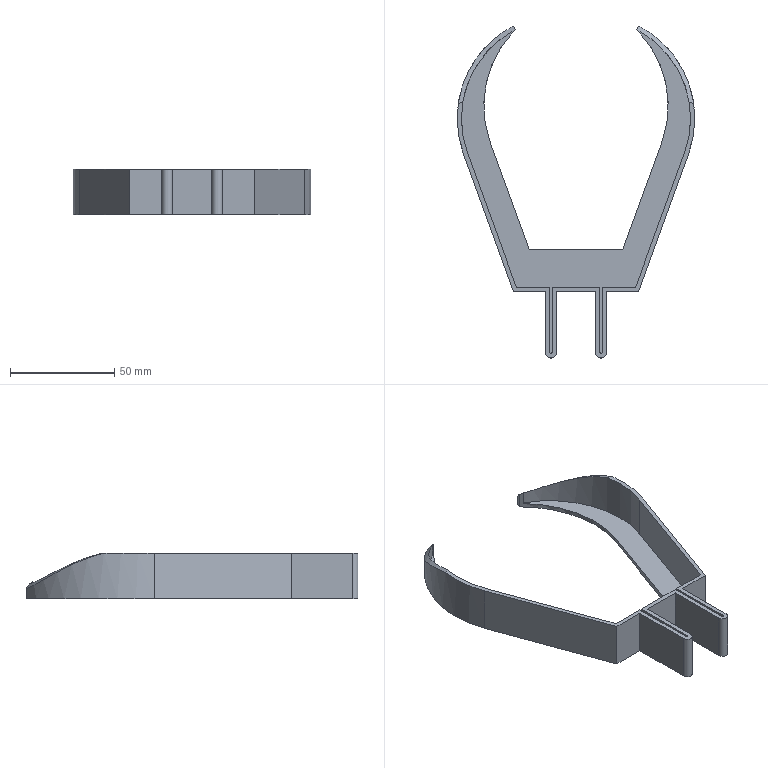Part | NX | features EXTRUDE 3, DATUM_CSYS 2, EXTRACT_STRING 2, SKETCH 2, Instance Feature 1, Mirror Feature 1, SHELL 1 | 1 solid | 40 faces | box 113.914 x 159.253 x 22 mm | volume 25744 mm3 | plane 28 | cylinder 12 | commonest cylinder face diameters 1 x2 5 x2 96 x2 100 x2 102.897 x2 103.017 x2
STEP:
#1=CARTESIAN_POINT('',(30.,127.253,4.945));
#2=VERTEX_POINT('',#1);
#3=CARTESIAN_POINT('',(29.078,125.478,7.237));
#4=VERTEX_POINT('',#3);
#5=CARTESIAN_POINT('',(11.445,91.523,-27.603));
#6=DIRECTION('',(-0.8875,0.4609,0.));
#7=DIRECTION('',(0.4609,0.8875,0.));
#8=AXIS2_PLACEMENT_3D('',#5,#6,#7);
#9=ELLIPSE('',#8,51.946,51.508);
#10=EDGE_CURVE('',#2,#4,#9,.F.);
#11=ORIENTED_EDGE('',*,*,#10,.F.);
#12=CARTESIAN_POINT('',(30.,127.253,0.));
#13=VERTEX_POINT('',#12);
#14=CARTESIAN_POINT('',(30.,127.253,22.));
#15=DIRECTION('',(0.,0.,-1.));
#16=VECTOR('',#15,1000.);
#17=LINE('',#14,#16);
#18=EDGE_CURVE('',#2,#13,#17,.T.);
#19=ORIENTED_EDGE('',*,*,#18,.T.);
#20=CARTESIAN_POINT('',(29.078,125.478,0.));
#21=VERTEX_POINT('',#20);
#22=CARTESIAN_POINT('',(29.078,125.478,0.));
#23=DIRECTION('',(0.4609,0.8875,0.));
#24=VECTOR('',#23,1000.);
#25=LINE('',#22,#24);
#26=EDGE_CURVE('',#21,#13,#25,.T.);
#27=ORIENTED_EDGE('',*,*,#26,.F.);
#28=CARTESIAN_POINT('',(29.078,125.478,22.));
#29=DIRECTION('',(0.,0.,-1.));
#30=VECTOR('',#29,1000.);
#31=LINE('',#28,#30);
#32=EDGE_CURVE('',#4,#21,#31,.T.);
#33=ORIENTED_EDGE('',*,*,#32,.F.);
#34=EDGE_LOOP('',(#11,#19,#27,#33));
#35=FACE_BOUND('',#34,.T.);
#36=CARTESIAN_POINT('',(29.078,125.478,22.));
#37=DIRECTION('',(-0.8875,0.4609,0.));
#38=DIRECTION('',(-0.4609,-0.8875,0.));
#39=AXIS2_PLACEMENT_3D('',#36,#37,#38);
#40=PLANE('',#39);
#41=ADVANCED_FACE('',(#35),#40,.T.);
#42=CARTESIAN_POINT('',(30.834,124.519,7.561));
#43=VERTEX_POINT('',#42);
#44=CARTESIAN_POINT('',(30.834,124.519,2.));
#45=VERTEX_POINT('',#44);
#46=CARTESIAN_POINT('',(30.834,124.519,22.));
#47=DIRECTION('',(0.,0.,-1.));
#48=VECTOR('',#47,1000.);
#49=LINE('',#46,#48);
#50=EDGE_CURVE('',#43,#45,#49,.T.);
#51=ORIENTED_EDGE('',*,*,#50,.F.);
#52=CARTESIAN_POINT('',(30.543,123.959,8.219));
#53=VERTEX_POINT('',#52);
#54=CARTESIAN_POINT('',(13.341,90.833,-27.603));
#55=DIRECTION('',(-0.8875,0.4609,0.));
#56=DIRECTION('',(0.4609,0.8875,0.));
#57=AXIS2_PLACEMENT_3D('',#54,#55,#56);
#58=ELLIPSE('',#57,51.946,51.508);
#59=EDGE_CURVE('',#43,#53,#58,.F.);
#60=ORIENTED_EDGE('',*,*,#59,.T.);
#61=CARTESIAN_POINT('',(30.543,123.959,2.));
#62=VERTEX_POINT('',#61);
#63=CARTESIAN_POINT('',(30.543,123.959,22.));
#64=DIRECTION('',(0.,0.,-1.));
#65=VECTOR('',#64,1000.);
#66=LINE('',#63,#65);
#67=EDGE_CURVE('',#53,#62,#66,.T.);
#68=ORIENTED_EDGE('',*,*,#67,.T.);
#69=CARTESIAN_POINT('',(5.777,76.267,2.));
#70=DIRECTION('',(0.4609,0.8875,0.));
#71=VECTOR('',#70,1000.);
#72=LINE('',#69,#71);
#73=EDGE_CURVE('',#62,#45,#72,.T.);
#74=ORIENTED_EDGE('',*,*,#73,.T.);
#75=EDGE_LOOP('',(#51,#60,#68,#74));
#76=FACE_BOUND('',#75,.T.);
#77=CARTESIAN_POINT('',(30.853,124.556,22.));
#78=DIRECTION('',(-0.8875,0.4609,0.));
#79=DIRECTION('',(-0.4609,-0.8875,0.));
#80=AXIS2_PLACEMENT_3D('',#77,#78,#79);
#81=PLANE('',#80);
#82=ADVANCED_FACE('',(#76),#81,.F.);
#83=CARTESIAN_POINT('',(-29.078,125.478,7.237));
#84=VERTEX_POINT('',#83);
#85=CARTESIAN_POINT('',(-30.,127.253,4.945));
#86=VERTEX_POINT('',#85);
#87=CARTESIAN_POINT('',(-11.445,91.523,-27.603));
#88=DIRECTION('',(0.8875,0.4609,0.));
#89=DIRECTION('',(-0.4609,0.8875,0.));
#90=AXIS2_PLACEMENT_3D('',#87,#88,#89);
#91=ELLIPSE('',#90,51.946,51.508);
#92=EDGE_CURVE('',#84,#86,#91,.F.);
#93=ORIENTED_EDGE('',*,*,#92,.F.);
#94=CARTESIAN_POINT('',(-29.078,125.478,0.));
#95=VERTEX_POINT('',#94);
#96=CARTESIAN_POINT('',(-29.078,125.478,22.));
#97=DIRECTION('',(0.,0.,-1.));
#98=VECTOR('',#97,1000.);
#99=LINE('',#96,#98);
#100=EDGE_CURVE('',#84,#95,#99,.T.);
#101=ORIENTED_EDGE('',*,*,#100,.T.);
#102=CARTESIAN_POINT('',(-30.,127.253,0.));
#103=VERTEX_POINT('',#102);
#104=CARTESIAN_POINT('',(-30.,127.253,0.));
#105=DIRECTION('',(0.4609,-0.8875,0.));
#106=VECTOR('',#105,1000.);
#107=LINE('',#104,#106);
#108=EDGE_CURVE('',#103,#95,#107,.T.);
#109=ORIENTED_EDGE('',*,*,#108,.F.);
#110=CARTESIAN_POINT('',(-30.,127.253,22.));
#111=DIRECTION('',(0.,0.,-1.));
#112=VECTOR('',#111,1000.);
#113=LINE('',#110,#112);
#114=EDGE_CURVE('',#86,#103,#113,.T.);
#115=ORIENTED_EDGE('',*,*,#114,.F.);
#116=EDGE_LOOP('',(#93,#101,#109,#115));
#117=FACE_BOUND('',#116,.T.);
#118=CARTESIAN_POINT('',(-30.,127.253,22.));
#119=DIRECTION('',(0.8875,0.4609,0.));
#120=DIRECTION('',(-0.4609,0.8875,0.));
#121=AXIS2_PLACEMENT_3D('',#118,#119,#120);
#122=PLANE('',#121);
#123=ADVANCED_FACE('',(#117),#122,.T.);
#124=CARTESIAN_POINT('',(-30.543,123.959,8.219));
#125=VERTEX_POINT('',#124);
#126=CARTESIAN_POINT('',(-30.543,123.959,2.));
#127=VERTEX_POINT('',#126);
#128=CARTESIAN_POINT('',(-30.543,123.959,22.));
#129=DIRECTION('',(0.,0.,-1.));
#130=VECTOR('',#129,1000.);
#131=LINE('',#128,#130);
#132=EDGE_CURVE('',#125,#127,#131,.T.);
#133=ORIENTED_EDGE('',*,*,#132,.F.);
#134=CARTESIAN_POINT('',(-30.834,124.519,7.561));
#135=VERTEX_POINT('',#134);
#136=CARTESIAN_POINT('',(-13.341,90.833,-27.603));
#137=DIRECTION('',(0.8875,0.4609,0.));
#138=DIRECTION('',(-0.4609,0.8875,0.));
#139=AXIS2_PLACEMENT_3D('',#136,#137,#138);
#140=ELLIPSE('',#139,51.946,51.508);
#141=EDGE_CURVE('',#125,#135,#140,.F.);
#142=ORIENTED_EDGE('',*,*,#141,.T.);
#143=CARTESIAN_POINT('',(-30.834,124.519,2.));
#144=VERTEX_POINT('',#143);
#145=CARTESIAN_POINT('',(-30.834,124.519,22.));
#146=DIRECTION('',(0.,0.,-1.));
#147=VECTOR('',#146,1000.);
#148=LINE('',#145,#147);
#149=EDGE_CURVE('',#135,#144,#148,.T.);
#150=ORIENTED_EDGE('',*,*,#149,.T.);
#151=CARTESIAN_POINT('',(-8.732,81.958,2.));
#152=DIRECTION('',(0.4609,-0.8875,0.));
#153=VECTOR('',#152,1000.);
#154=LINE('',#151,#153);
#155=EDGE_CURVE('',#144,#127,#154,.T.);
#156=ORIENTED_EDGE('',*,*,#155,.T.);
#157=EDGE_LOOP('',(#133,#142,#150,#156));
#158=FACE_BOUND('',#157,.T.);
#159=CARTESIAN_POINT('',(-31.775,126.331,22.));
#160=DIRECTION('',(0.8875,0.4609,0.));
#161=DIRECTION('',(-0.4609,0.8875,0.));
#162=AXIS2_PLACEMENT_3D('',#159,#160,#161);
#163=PLANE('',#162);
#164=ADVANCED_FACE('',(#158),#163,.F.);
#165=CARTESIAN_POINT('',(-30.543,123.959,8.219));
#166=CARTESIAN_POINT('',(-30.068,124.473,7.889));
#167=CARTESIAN_POINT('',(-29.58,124.979,7.561));
#168=CARTESIAN_POINT('',(-29.078,125.478,7.237));
#169=B_SPLINE_CURVE_WITH_KNOTS('',3,(#165,#166,#167,#168),.UNSPECIFIED.,.F.,.F.,(4,4),(0.0356,0.0379),.UNSPECIFIED.);
#170=EDGE_CURVE('',#125,#84,#169,.T.);
#171=ORIENTED_EDGE('',*,*,#170,.F.);
#172=ORIENTED_EDGE('',*,*,#132,.T.);
#173=CARTESIAN_POINT('',(-41.696,73.068,2.));
#174=VERTEX_POINT('',#173);
#175=CARTESIAN_POINT('',(7.219,89.016,2.));
#176=DIRECTION('',(0.,0.,-1.));
#177=DIRECTION('',(-1.,0.,0.));
#178=AXIS2_PLACEMENT_3D('',#175,#176,#177);
#179=CIRCLE('',#178,51.449);
#180=EDGE_CURVE('',#127,#174,#179,.F.);
#181=ORIENTED_EDGE('',*,*,#180,.T.);
#182=CARTESIAN_POINT('',(-41.696,73.068,0.));
#183=VERTEX_POINT('',#182);
#184=CARTESIAN_POINT('',(-41.696,73.068,22.));
#185=DIRECTION('',(0.,0.,-1.));
#186=VECTOR('',#185,1000.);
#187=LINE('',#184,#186);
#188=EDGE_CURVE('',#174,#183,#187,.T.);
#189=ORIENTED_EDGE('',*,*,#188,.T.);
#190=CARTESIAN_POINT('',(7.219,89.016,0.));
#191=DIRECTION('',(0.,0.,1.));
#192=DIRECTION('',(-1.,0.,0.));
#193=AXIS2_PLACEMENT_3D('',#190,#191,#192);
#194=CIRCLE('',#193,51.449);
#195=EDGE_CURVE('',#95,#183,#194,.T.);
#196=ORIENTED_EDGE('',*,*,#195,.F.);
#197=ORIENTED_EDGE('',*,*,#100,.F.);
#198=EDGE_LOOP('',(#171,#172,#181,#189,#196,#197));
#199=FACE_BOUND('',#198,.T.);
#200=CARTESIAN_POINT('',(7.219,89.016,22.));
#201=DIRECTION('',(0.,0.,-1.));
#202=DIRECTION('',(-1.,0.,0.));
#203=AXIS2_PLACEMENT_3D('',#200,#201,#202);
#204=CYLINDRICAL_SURFACE('',#203,51.449);
#205=ADVANCED_FACE('',(#199),#204,.F.);
#206=ORIENTED_EDGE('',*,*,#188,.F.);
#207=CARTESIAN_POINT('',(-22.381,20.,2.));
#208=VERTEX_POINT('',#207);
#209=CARTESIAN_POINT('',(-40.786,70.567,2.));
#210=DIRECTION('',(0.342,-0.9397,0.));
#211=VECTOR('',#210,1000.);
#212=LINE('',#209,#211);
#213=EDGE_CURVE('',#174,#208,#212,.T.);
#214=ORIENTED_EDGE('',*,*,#213,.T.);
#215=CARTESIAN_POINT('',(-22.381,20.,0.));
#216=VERTEX_POINT('',#215);
#217=CARTESIAN_POINT('',(-22.381,20.,22.));
#218=DIRECTION('',(0.,0.,-1.));
#219=VECTOR('',#218,1000.);
#220=LINE('',#217,#219);
#221=EDGE_CURVE('',#208,#216,#220,.T.);
#222=ORIENTED_EDGE('',*,*,#221,.T.);
#223=CARTESIAN_POINT('',(-41.696,73.068,0.));
#224=DIRECTION('',(0.342,-0.9397,0.));
#225=VECTOR('',#224,1000.);
#226=LINE('',#223,#225);
#227=EDGE_CURVE('',#183,#216,#226,.T.);
#228=ORIENTED_EDGE('',*,*,#227,.F.);
#229=EDGE_LOOP('',(#206,#214,#222,#228));
#230=FACE_BOUND('',#229,.T.);
#231=CARTESIAN_POINT('',(-41.696,73.068,22.));
#232=DIRECTION('',(0.9397,0.342,0.));
#233=DIRECTION('',(-0.342,0.9397,0.));
#234=AXIS2_PLACEMENT_3D('',#231,#232,#233);
#235=PLANE('',#234);
#236=ADVANCED_FACE('',(#230),#235,.T.);
#237=ORIENTED_EDGE('',*,*,#221,.F.);
#238=CARTESIAN_POINT('',(22.381,20.,2.));
#239=VERTEX_POINT('',#238);
#240=CARTESIAN_POINT('',(-6.957,20.,2.));
#241=DIRECTION('',(1.,0.,0.));
#242=VECTOR('',#241,1000.);
#243=LINE('',#240,#242);
#244=EDGE_CURVE('',#208,#239,#243,.T.);
#245=ORIENTED_EDGE('',*,*,#244,.T.);
#246=CARTESIAN_POINT('',(22.381,20.,0.));
#247=VERTEX_POINT('',#246);
#248=CARTESIAN_POINT('',(22.381,20.,22.));
#249=DIRECTION('',(0.,0.,-1.));
#250=VECTOR('',#249,1000.);
#251=LINE('',#248,#250);
#252=EDGE_CURVE('',#239,#247,#251,.T.);
#253=ORIENTED_EDGE('',*,*,#252,.T.);
#254=CARTESIAN_POINT('',(-22.381,20.,0.));
#255=DIRECTION('',(1.,0.,0.));
#256=VECTOR('',#255,1000.);
#257=LINE('',#254,#256);
#258=EDGE_CURVE('',#216,#247,#257,.T.);
#259=ORIENTED_EDGE('',*,*,#258,.F.);
#260=EDGE_LOOP('',(#237,#245,#253,#259));
#261=FACE_BOUND('',#260,.T.);
#262=CARTESIAN_POINT('',(-22.381,20.,22.));
#263=DIRECTION('',(0.,1.,0.));
#264=DIRECTION('',(0.,0.,1.));
#265=AXIS2_PLACEMENT_3D('',#262,#263,#264);
#266=PLANE('',#265);
#267=ADVANCED_FACE('',(#261),#266,.T.);
#268=ORIENTED_EDGE('',*,*,#252,.F.);
#269=CARTESIAN_POINT('',(41.696,73.068,2.));
#270=VERTEX_POINT('',#269);
#271=CARTESIAN_POINT('',(39.158,66.095,2.));
#272=DIRECTION('',(0.342,0.9397,0.));
#273=VECTOR('',#272,1000.);
#274=LINE('',#271,#273);
#275=EDGE_CURVE('',#239,#270,#274,.T.);
#276=ORIENTED_EDGE('',*,*,#275,.T.);
#277=CARTESIAN_POINT('',(41.696,73.068,0.));
#278=VERTEX_POINT('',#277);
#279=CARTESIAN_POINT('',(41.696,73.068,22.));
#280=DIRECTION('',(0.,0.,-1.));
#281=VECTOR('',#280,1000.);
#282=LINE('',#279,#281);
#283=EDGE_CURVE('',#270,#278,#282,.T.);
#284=ORIENTED_EDGE('',*,*,#283,.T.);
#285=CARTESIAN_POINT('',(22.381,20.,0.));
#286=DIRECTION('',(0.342,0.9397,0.));
#287=VECTOR('',#286,1000.);
#288=LINE('',#285,#287);
#289=EDGE_CURVE('',#247,#278,#288,.T.);
#290=ORIENTED_EDGE('',*,*,#289,.F.);
#291=EDGE_LOOP('',(#268,#276,#284,#290));
#292=FACE_BOUND('',#291,.T.);
#293=CARTESIAN_POINT('',(22.381,20.,22.));
#294=DIRECTION('',(-0.9397,0.342,0.));
#295=DIRECTION('',(-0.342,-0.9397,0.));
#296=AXIS2_PLACEMENT_3D('',#293,#294,#295);
#297=PLANE('',#296);
#298=ADVANCED_FACE('',(#292),#297,.T.);
#299=CARTESIAN_POINT('',(29.078,125.478,7.237));
#300=CARTESIAN_POINT('',(29.58,124.979,7.561));
#301=CARTESIAN_POINT('',(30.068,124.473,7.889));
#302=CARTESIAN_POINT('',(30.543,123.959,8.219));
#303=B_SPLINE_CURVE_WITH_KNOTS('',3,(#299,#300,#301,#302),.UNSPECIFIED.,.F.,.F.,(4,4),(0.,0.002303),.UNSPECIFIED.);
#304=EDGE_CURVE('',#4,#53,#303,.T.);
#305=ORIENTED_EDGE('',*,*,#304,.F.);
#306=ORIENTED_EDGE('',*,*,#32,.T.);
#307=CARTESIAN_POINT('',(-7.219,89.016,0.));
#308=DIRECTION('',(0.,0.,1.));
#309=DIRECTION('',(1.,0.,0.));
#310=AXIS2_PLACEMENT_3D('',#307,#308,#309);
#311=CIRCLE('',#310,51.449);
#312=EDGE_CURVE('',#278,#21,#311,.T.);
#313=ORIENTED_EDGE('',*,*,#312,.F.);
#314=ORIENTED_EDGE('',*,*,#283,.F.);
#315=CARTESIAN_POINT('',(-7.219,89.016,2.));
#316=DIRECTION('',(0.,0.,-1.));
#317=DIRECTION('',(-1.,0.,0.));
#318=AXIS2_PLACEMENT_3D('',#315,#316,#317);
#319=CIRCLE('',#318,51.449);
#320=EDGE_CURVE('',#270,#62,#319,.F.);
#321=ORIENTED_EDGE('',*,*,#320,.T.);
#322=ORIENTED_EDGE('',*,*,#67,.F.);
#323=EDGE_LOOP('',(#305,#306,#313,#314,#321,#322));
#324=FACE_BOUND('',#323,.T.);
#325=CARTESIAN_POINT('',(-7.219,89.016,22.));
#326=DIRECTION('',(0.,0.,-1.));
#327=DIRECTION('',(-1.,0.,0.));
#328=AXIS2_PLACEMENT_3D('',#325,#326,#327);
#329=CYLINDRICAL_SURFACE('',#328,51.449);
#330=ADVANCED_FACE('',(#324),#329,.F.);
#331=CARTESIAN_POINT('',(-56.46,89.91,22.));
#332=VERTEX_POINT('',#331);
#333=CARTESIAN_POINT('',(-30.,127.253,4.945));
#334=CARTESIAN_POINT('',(-33.752,125.305,5.617));
#335=CARTESIAN_POINT('',(-38.676,121.879,7.46));
#336=CARTESIAN_POINT('',(-44.283,116.32,10.676));
#337=CARTESIAN_POINT('',(-47.878,111.8,13.209));
#338=CARTESIAN_POINT('',(-50.929,106.918,15.731));
#339=CARTESIAN_POINT('',(-54.297,99.795,18.969));
#340=CARTESIAN_POINT('',(-55.878,94.006,20.979));
#341=CARTESIAN_POINT('',(-56.46,89.91,22.));
#342=B_SPLINE_CURVE_WITH_KNOTS('',3,(#333,#334,#335,#336,#337,#338,#339,#340,#341),.UNSPECIFIED.,.F.,.F.,(4,1,1,1,1,1,4),(0.,0.01257,0.01885,0.02514,0.03142,0.03771,0.05028),.UNSPECIFIED.);
#343=EDGE_CURVE('',#86,#332,#342,.T.);
#344=ORIENTED_EDGE('',*,*,#343,.F.);
#345=ORIENTED_EDGE('',*,*,#114,.T.);
#346=CARTESIAN_POINT('',(-53.941,65.778,0.));
#347=VERTEX_POINT('',#346);
#348=CARTESIAN_POINT('',(-6.957,82.879,0.));
#349=DIRECTION('',(0.,0.,-1.));
#350=DIRECTION('',(-1.,0.,0.));
#351=AXIS2_PLACEMENT_3D('',#348,#349,#350);
#352=CIRCLE('',#351,50.);
#353=EDGE_CURVE('',#347,#103,#352,.T.);
#354=ORIENTED_EDGE('',*,*,#353,.F.);
#355=CARTESIAN_POINT('',(-53.941,65.778,22.));
#356=VERTEX_POINT('',#355);
#357=CARTESIAN_POINT('',(-53.941,65.778,22.));
#358=DIRECTION('',(0.,0.,-1.));
#359=VECTOR('',#358,1000.);
#360=LINE('',#357,#359);
#361=EDGE_CURVE('',#356,#347,#360,.T.);
#362=ORIENTED_EDGE('',*,*,#361,.F.);
#363=CARTESIAN_POINT('',(-6.957,82.879,22.));
#364=DIRECTION('',(0.,0.,-1.));
#365=DIRECTION('',(-0.9397,-0.342,0.));
#366=AXIS2_PLACEMENT_3D('',#363,#364,#365);
#367=CIRCLE('',#366,50.);
#368=EDGE_CURVE('',#356,#332,#367,.T.);
#369=ORIENTED_EDGE('',*,*,#368,.T.);
#370=EDGE_LOOP('',(#344,#345,#354,#362,#369));
#371=FACE_BOUND('',#370,.T.);
#372=CARTESIAN_POINT('',(-6.957,82.879,22.));
#373=DIRECTION('',(0.,0.,-1.));
#374=DIRECTION('',(-1.,0.,0.));
#375=AXIS2_PLACEMENT_3D('',#372,#373,#374);
#376=CYLINDRICAL_SURFACE('',#375,50.);
#377=ADVANCED_FACE('',(#371),#376,.T.);
#378=CARTESIAN_POINT('',(56.46,89.91,22.));
#379=VERTEX_POINT('',#378);
#380=CARTESIAN_POINT('',(56.46,89.91,22.));
#381=CARTESIAN_POINT('',(55.878,94.009,20.978));
#382=CARTESIAN_POINT('',(53.783,101.68,18.316));
#383=CARTESIAN_POINT('',(49.082,110.291,14.057));
#384=CARTESIAN_POINT('',(44.296,116.303,10.685));
#385=CARTESIAN_POINT('',(38.69,121.87,7.465));
#386=CARTESIAN_POINT('',(33.748,125.307,5.616));
#387=CARTESIAN_POINT('',(30.,127.253,4.945));
#388=B_SPLINE_CURVE_WITH_KNOTS('',3,(#380,#381,#382,#383,#384,#385,#386,#387),.UNSPECIFIED.,.F.,.F.,(4,1,1,1,1,4),(0.,0.01257,0.02515,0.03144,0.03772,0.0503),.UNSPECIFIED.);
#389=EDGE_CURVE('',#379,#2,#388,.T.);
#390=ORIENTED_EDGE('',*,*,#389,.F.);
#391=CARTESIAN_POINT('',(53.941,65.778,22.));
#392=VERTEX_POINT('',#391);
#393=CARTESIAN_POINT('',(6.957,82.879,22.));
#394=DIRECTION('',(0.,0.,-1.));
#395=DIRECTION('',(0.4609,0.8875,0.));
#396=AXIS2_PLACEMENT_3D('',#393,#394,#395);
#397=CIRCLE('',#396,50.);
#398=EDGE_CURVE('',#379,#392,#397,.T.);
#399=ORIENTED_EDGE('',*,*,#398,.T.);
#400=CARTESIAN_POINT('',(53.941,65.778,0.));
#401=VERTEX_POINT('',#400);
#402=CARTESIAN_POINT('',(53.941,65.778,22.));
#403=DIRECTION('',(0.,0.,-1.));
#404=VECTOR('',#403,1000.);
#405=LINE('',#402,#404);
#406=EDGE_CURVE('',#392,#401,#405,.T.);
#407=ORIENTED_EDGE('',*,*,#406,.T.);
#408=CARTESIAN_POINT('',(6.957,82.879,0.));
#409=DIRECTION('',(0.,0.,-1.));
#410=DIRECTION('',(1.,0.,0.));
#411=AXIS2_PLACEMENT_3D('',#408,#409,#410);
#412=CIRCLE('',#411,50.);
#413=EDGE_CURVE('',#13,#401,#412,.T.);
#414=ORIENTED_EDGE('',*,*,#413,.F.);
#415=ORIENTED_EDGE('',*,*,#18,.F.);
#416=EDGE_LOOP('',(#390,#399,#407,#414,#415));
#417=FACE_BOUND('',#416,.T.);
#418=CARTESIAN_POINT('',(6.957,82.879,22.));
#419=DIRECTION('',(0.,0.,-1.));
#420=DIRECTION('',(-1.,0.,0.));
#421=AXIS2_PLACEMENT_3D('',#418,#419,#420);
#422=CYLINDRICAL_SURFACE('',#421,50.);
#423=ADVANCED_FACE('',(#417),#422,.T.);
#424=CARTESIAN_POINT('',(30.,0.,0.));
#425=VERTEX_POINT('',#424);
#426=CARTESIAN_POINT('',(53.941,65.778,0.));
#427=DIRECTION('',(-0.342,-0.9397,0.));
#428=VECTOR('',#427,1000.);
#429=LINE('',#426,#428);
#430=EDGE_CURVE('',#401,#425,#429,.T.);
#431=ORIENTED_EDGE('',*,*,#430,.F.);
#432=ORIENTED_EDGE('',*,*,#406,.F.);
#433=CARTESIAN_POINT('',(30.,0.,22.));
#434=VERTEX_POINT('',#433);
#435=CARTESIAN_POINT('',(53.941,65.778,22.));
#436=DIRECTION('',(-0.342,-0.9397,0.));
#437=VECTOR('',#436,1000.);
#438=LINE('',#435,#437);
#439=EDGE_CURVE('',#392,#434,#438,.T.);
#440=ORIENTED_EDGE('',*,*,#439,.T.);
#441=CARTESIAN_POINT('',(30.,0.,22.));
#442=DIRECTION('',(0.,0.,-1.));
#443=VECTOR('',#442,1000.);
#444=LINE('',#441,#443);
#445=EDGE_CURVE('',#434,#425,#444,.T.);
#446=ORIENTED_EDGE('',*,*,#445,.T.);
#447=EDGE_LOOP('',(#431,#432,#440,#446));
#448=FACE_BOUND('',#447,.T.);
#449=CARTESIAN_POINT('',(53.941,65.778,22.));
#450=DIRECTION('',(0.9397,-0.342,0.));
#451=DIRECTION('',(0.342,0.9397,0.));
#452=AXIS2_PLACEMENT_3D('',#449,#450,#451);
#453=PLANE('',#452);
#454=ADVANCED_FACE('',(#448),#453,.T.);
#455=CARTESIAN_POINT('',(14.5,0.,0.));
#456=VERTEX_POINT('',#455);
#457=CARTESIAN_POINT('',(30.,0.,0.));
#458=DIRECTION('',(-1.,0.,0.));
#459=VECTOR('',#458,1000.);
#460=LINE('',#457,#459);
#461=EDGE_CURVE('',#425,#456,#460,.T.);
#462=ORIENTED_EDGE('',*,*,#461,.F.);
#463=ORIENTED_EDGE('',*,*,#445,.F.);
#464=CARTESIAN_POINT('',(14.5,0.,22.));
#465=VERTEX_POINT('',#464);
#466=CARTESIAN_POINT('',(30.,0.,22.));
#467=DIRECTION('',(-1.,0.,0.));
#468=VECTOR('',#467,1000.);
#469=LINE('',#466,#468);
#470=EDGE_CURVE('',#434,#465,#469,.T.);
#471=ORIENTED_EDGE('',*,*,#470,.T.);
#472=CARTESIAN_POINT('',(14.5,0.,22.));
#473=DIRECTION('',(0.,0.,-1.));
#474=VECTOR('',#473,1000.);
#475=LINE('',#472,#474);
#476=EDGE_CURVE('',#465,#456,#475,.T.);
#477=ORIENTED_EDGE('',*,*,#476,.T.);
#478=EDGE_LOOP('',(#462,#463,#471,#477));
#479=FACE_BOUND('',#478,.T.);
#480=CARTESIAN_POINT('',(30.,0.,22.));
#481=DIRECTION('',(0.,-1.,0.));
#482=DIRECTION('',(0.,0.,-1.));
#483=AXIS2_PLACEMENT_3D('',#480,#481,#482);
#484=PLANE('',#483);
#485=ADVANCED_FACE('',(#479),#484,.T.);
#486=CARTESIAN_POINT('',(14.5,-29.5,0.));
#487=VERTEX_POINT('',#486);
#488=CARTESIAN_POINT('',(14.5,0.,0.));
#489=DIRECTION('',(0.,-1.,0.));
#490=VECTOR('',#489,1000.);
#491=LINE('',#488,#490);
#492=EDGE_CURVE('',#456,#487,#491,.T.);
#493=ORIENTED_EDGE('',*,*,#492,.F.);
#494=ORIENTED_EDGE('',*,*,#476,.F.);
#495=CARTESIAN_POINT('',(14.5,-29.5,22.));
#496=VERTEX_POINT('',#495);
#497=CARTESIAN_POINT('',(14.5,0.,22.));
#498=DIRECTION('',(0.,-1.,0.));
#499=VECTOR('',#498,1000.);
#500=LINE('',#497,#499);
#501=EDGE_CURVE('',#465,#496,#500,.T.);
#502=ORIENTED_EDGE('',*,*,#501,.T.);
#503=CARTESIAN_POINT('',(14.5,-29.5,22.));
#504=DIRECTION('',(0.,0.,-1.));
#505=VECTOR('',#504,1000.);
#506=LINE('',#503,#505);
#507=EDGE_CURVE('',#496,#487,#506,.T.);
#508=ORIENTED_EDGE('',*,*,#507,.T.);
#509=EDGE_LOOP('',(#493,#494,#502,#508));
#510=FACE_BOUND('',#509,.T.);
#511=CARTESIAN_POINT('',(14.5,0.,22.));
#512=DIRECTION('',(1.,0.,0.));
#513=DIRECTION('',(0.,0.,-1.));
#514=AXIS2_PLACEMENT_3D('',#511,#512,#513);
#515=PLANE('',#514);
#516=ADVANCED_FACE('',(#510),#515,.T.);
#517=CARTESIAN_POINT('',(9.5,-29.5,0.));
#518=VERTEX_POINT('',#517);
#519=CARTESIAN_POINT('',(12.,-29.5,0.));
#520=DIRECTION('',(0.,0.,-1.));
#521=DIRECTION('',(1.,0.,0.));
#522=AXIS2_PLACEMENT_3D('',#519,#520,#521);
#523=CIRCLE('',#522,2.5);
#524=EDGE_CURVE('',#487,#518,#523,.T.);
#525=ORIENTED_EDGE('',*,*,#524,.F.);
#526=ORIENTED_EDGE('',*,*,#507,.F.);
#527=CARTESIAN_POINT('',(9.5,-29.5,22.));
#528=VERTEX_POINT('',#527);
#529=CARTESIAN_POINT('',(12.,-29.5,22.));
#530=DIRECTION('',(0.,0.,-1.));
#531=DIRECTION('',(1.,0.,0.));
#532=AXIS2_PLACEMENT_3D('',#529,#530,#531);
#533=CIRCLE('',#532,2.5);
#534=EDGE_CURVE('',#496,#528,#533,.T.);
#535=ORIENTED_EDGE('',*,*,#534,.T.);
#536=CARTESIAN_POINT('',(9.5,-29.5,22.));
#537=DIRECTION('',(0.,0.,-1.));
#538=VECTOR('',#537,1000.);
#539=LINE('',#536,#538);
#540=EDGE_CURVE('',#528,#518,#539,.T.);
#541=ORIENTED_EDGE('',*,*,#540,.T.);
#542=EDGE_LOOP('',(#525,#526,#535,#541));
#543=FACE_BOUND('',#542,.T.);
#544=CARTESIAN_POINT('',(12.,-29.5,22.));
#545=DIRECTION('',(0.,0.,-1.));
#546=DIRECTION('',(-1.,0.,0.));
#547=AXIS2_PLACEMENT_3D('',#544,#545,#546);
#548=CYLINDRICAL_SURFACE('',#547,2.5);
#549=ADVANCED_FACE('',(#543),#548,.T.);
#550=CARTESIAN_POINT('',(9.5,0.,0.));
#551=VERTEX_POINT('',#550);
#552=CARTESIAN_POINT('',(9.5,-29.5,0.));
#553=DIRECTION('',(0.,1.,0.));
#554=VECTOR('',#553,1000.);
#555=LINE('',#552,#554);
#556=EDGE_CURVE('',#518,#551,#555,.T.);
#557=ORIENTED_EDGE('',*,*,#556,.F.);
#558=ORIENTED_EDGE('',*,*,#540,.F.);
#559=CARTESIAN_POINT('',(9.5,0.,22.));
#560=VERTEX_POINT('',#559);
#561=CARTESIAN_POINT('',(9.5,-29.5,22.));
#562=DIRECTION('',(0.,1.,0.));
#563=VECTOR('',#562,1000.);
#564=LINE('',#561,#563);
#565=EDGE_CURVE('',#528,#560,#564,.T.);
#566=ORIENTED_EDGE('',*,*,#565,.T.);
#567=CARTESIAN_POINT('',(9.5,0.,22.));
#568=DIRECTION('',(0.,0.,-1.));
#569=VECTOR('',#568,1000.);
#570=LINE('',#567,#569);
#571=EDGE_CURVE('',#560,#551,#570,.T.);
#572=ORIENTED_EDGE('',*,*,#571,.T.);
#573=EDGE_LOOP('',(#557,#558,#566,#572));
#574=FACE_BOUND('',#573,.T.);
#575=CARTESIAN_POINT('',(9.5,-29.5,22.));
#576=DIRECTION('',(-1.,0.,0.));
#577=DIRECTION('',(0.,0.,1.));
#578=AXIS2_PLACEMENT_3D('',#575,#576,#577);
#579=PLANE('',#578);
#580=ADVANCED_FACE('',(#574),#579,.T.);
#581=CARTESIAN_POINT('',(-9.5,0.,0.));
#582=VERTEX_POINT('',#581);
#583=CARTESIAN_POINT('',(9.5,0.,0.));
#584=DIRECTION('',(-1.,0.,0.));
#585=VECTOR('',#584,1000.);
#586=LINE('',#583,#585);
#587=EDGE_CURVE('',#551,#582,#586,.T.);
#588=ORIENTED_EDGE('',*,*,#587,.F.);
#589=ORIENTED_EDGE('',*,*,#571,.F.);
#590=CARTESIAN_POINT('',(-9.5,0.,22.));
#591=VERTEX_POINT('',#590);
#592=CARTESIAN_POINT('',(9.5,0.,22.));
#593=DIRECTION('',(-1.,0.,0.));
#594=VECTOR('',#593,1000.);
#595=LINE('',#592,#594);
#596=EDGE_CURVE('',#560,#591,#595,.T.);
#597=ORIENTED_EDGE('',*,*,#596,.T.);
#598=CARTESIAN_POINT('',(-9.5,0.,22.));
#599=DIRECTION('',(0.,0.,-1.));
#600=VECTOR('',#599,1000.);
#601=LINE('',#598,#600);
#602=EDGE_CURVE('',#591,#582,#601,.T.);
#603=ORIENTED_EDGE('',*,*,#602,.T.);
#604=EDGE_LOOP('',(#588,#589,#597,#603));
#605=FACE_BOUND('',#604,.T.);
#606=CARTESIAN_POINT('',(9.5,0.,22.));
#607=DIRECTION('',(0.,-1.,0.));
#608=DIRECTION('',(0.,0.,-1.));
#609=AXIS2_PLACEMENT_3D('',#606,#607,#608);
#610=PLANE('',#609);
#611=ADVANCED_FACE('',(#605),#610,.T.);
#612=CARTESIAN_POINT('',(-9.5,-29.5,0.));
#613=VERTEX_POINT('',#612);
#614=CARTESIAN_POINT('',(-9.5,0.,0.));
#615=DIRECTION('',(0.,-1.,0.));
#616=VECTOR('',#615,1000.);
#617=LINE('',#614,#616);
#618=EDGE_CURVE('',#582,#613,#617,.T.);
#619=ORIENTED_EDGE('',*,*,#618,.F.);
#620=ORIENTED_EDGE('',*,*,#602,.F.);
#621=CARTESIAN_POINT('',(-9.5,-29.5,22.));
#622=VERTEX_POINT('',#621);
#623=CARTESIAN_POINT('',(-9.5,0.,22.));
#624=DIRECTION('',(0.,-1.,0.));
#625=VECTOR('',#624,1000.);
#626=LINE('',#623,#625);
#627=EDGE_CURVE('',#591,#622,#626,.T.);
#628=ORIENTED_EDGE('',*,*,#627,.T.);
#629=CARTESIAN_POINT('',(-9.5,-29.5,22.));
#630=DIRECTION('',(0.,0.,-1.));
#631=VECTOR('',#630,1000.);
#632=LINE('',#629,#631);
#633=EDGE_CURVE('',#622,#613,#632,.T.);
#634=ORIENTED_EDGE('',*,*,#633,.T.);
#635=EDGE_LOOP('',(#619,#620,#628,#634));
#636=FACE_BOUND('',#635,.T.);
#637=CARTESIAN_POINT('',(-9.5,0.,22.));
#638=DIRECTION('',(1.,0.,0.));
#639=DIRECTION('',(0.,0.,-1.));
#640=AXIS2_PLACEMENT_3D('',#637,#638,#639);
#641=PLANE('',#640);
#642=ADVANCED_FACE('',(#636),#641,.T.);
#643=CARTESIAN_POINT('',(-14.5,-29.5,0.));
#644=VERTEX_POINT('',#643);
#645=CARTESIAN_POINT('',(-12.,-29.5,0.));
#646=DIRECTION('',(0.,0.,-1.));
#647=DIRECTION('',(1.,0.,0.));
#648=AXIS2_PLACEMENT_3D('',#645,#646,#647);
#649=CIRCLE('',#648,2.5);
#650=EDGE_CURVE('',#613,#644,#649,.T.);
#651=ORIENTED_EDGE('',*,*,#650,.F.);
#652=ORIENTED_EDGE('',*,*,#633,.F.);
#653=CARTESIAN_POINT('',(-14.5,-29.5,22.));
#654=VERTEX_POINT('',#653);
#655=CARTESIAN_POINT('',(-12.,-29.5,22.));
#656=DIRECTION('',(0.,0.,-1.));
#657=DIRECTION('',(1.,0.,0.));
#658=AXIS2_PLACEMENT_3D('',#655,#656,#657);
#659=CIRCLE('',#658,2.5);
#660=EDGE_CURVE('',#622,#654,#659,.T.);
#661=ORIENTED_EDGE('',*,*,#660,.T.);
#662=CARTESIAN_POINT('',(-14.5,-29.5,22.));
#663=DIRECTION('',(0.,0.,-1.));
#664=VECTOR('',#663,1000.);
#665=LINE('',#662,#664);
#666=EDGE_CURVE('',#654,#644,#665,.T.);
#667=ORIENTED_EDGE('',*,*,#666,.T.);
#668=EDGE_LOOP('',(#651,#652,#661,#667));
#669=FACE_BOUND('',#668,.T.);
#670=CARTESIAN_POINT('',(-12.,-29.5,22.));
#671=DIRECTION('',(0.,0.,-1.));
#672=DIRECTION('',(-1.,0.,0.));
#673=AXIS2_PLACEMENT_3D('',#670,#671,#672);
#674=CYLINDRICAL_SURFACE('',#673,2.5);
#675=ADVANCED_FACE('',(#669),#674,.T.);
#676=CARTESIAN_POINT('',(-14.5,0.,0.));
#677=VERTEX_POINT('',#676);
#678=CARTESIAN_POINT('',(-14.5,-29.5,0.));
#679=DIRECTION('',(0.,1.,0.));
#680=VECTOR('',#679,1000.);
#681=LINE('',#678,#680);
#682=EDGE_CURVE('',#644,#677,#681,.T.);
#683=ORIENTED_EDGE('',*,*,#682,.F.);
#684=ORIENTED_EDGE('',*,*,#666,.F.);
#685=CARTESIAN_POINT('',(-14.5,0.,22.));
#686=VERTEX_POINT('',#685);
#687=CARTESIAN_POINT('',(-14.5,-29.5,22.));
#688=DIRECTION('',(0.,1.,0.));
#689=VECTOR('',#688,1000.);
#690=LINE('',#687,#689);
#691=EDGE_CURVE('',#654,#686,#690,.T.);
#692=ORIENTED_EDGE('',*,*,#691,.T.);
#693=CARTESIAN_POINT('',(-14.5,0.,22.));
#694=DIRECTION('',(0.,0.,-1.));
#695=VECTOR('',#694,1000.);
#696=LINE('',#693,#695);
#697=EDGE_CURVE('',#686,#677,#696,.T.);
#698=ORIENTED_EDGE('',*,*,#697,.T.);
#699=EDGE_LOOP('',(#683,#684,#692,#698));
#700=FACE_BOUND('',#699,.T.);
#701=CARTESIAN_POINT('',(-14.5,-29.5,22.));
#702=DIRECTION('',(-1.,0.,0.));
#703=DIRECTION('',(0.,0.,1.));
#704=AXIS2_PLACEMENT_3D('',#701,#702,#703);
#705=PLANE('',#704);
#706=ADVANCED_FACE('',(#700),#705,.T.);
#707=CARTESIAN_POINT('',(-30.,0.,0.));
#708=VERTEX_POINT('',#707);
#709=CARTESIAN_POINT('',(-14.5,0.,0.));
#710=DIRECTION('',(-1.,0.,0.));
#711=VECTOR('',#710,1000.);
#712=LINE('',#709,#711);
#713=EDGE_CURVE('',#677,#708,#712,.T.);
#714=ORIENTED_EDGE('',*,*,#713,.F.);
#715=ORIENTED_EDGE('',*,*,#697,.F.);
#716=CARTESIAN_POINT('',(-30.,0.,22.));
#717=VERTEX_POINT('',#716);
#718=CARTESIAN_POINT('',(-14.5,0.,22.));
#719=DIRECTION('',(-1.,0.,0.));
#720=VECTOR('',#719,1000.);
#721=LINE('',#718,#720);
#722=EDGE_CURVE('',#686,#717,#721,.T.);
#723=ORIENTED_EDGE('',*,*,#722,.T.);
#724=CARTESIAN_POINT('',(-30.,0.,22.));
#725=DIRECTION('',(0.,0.,-1.));
#726=VECTOR('',#725,1000.);
#727=LINE('',#724,#726);
#728=EDGE_CURVE('',#717,#708,#727,.T.);
#729=ORIENTED_EDGE('',*,*,#728,.T.);
#730=EDGE_LOOP('',(#714,#715,#723,#729));
#731=FACE_BOUND('',#730,.T.);
#732=CARTESIAN_POINT('',(-14.5,0.,22.));
#733=DIRECTION('',(0.,-1.,0.));
#734=DIRECTION('',(0.,0.,-1.));
#735=AXIS2_PLACEMENT_3D('',#732,#733,#734);
#736=PLANE('',#735);
#737=ADVANCED_FACE('',(#731),#736,.T.);
#738=CARTESIAN_POINT('',(-30.,0.,0.));
#739=DIRECTION('',(-0.342,0.9397,0.));
#740=VECTOR('',#739,1000.);
#741=LINE('',#738,#740);
#742=EDGE_CURVE('',#708,#347,#741,.T.);
#743=ORIENTED_EDGE('',*,*,#742,.F.);
#744=ORIENTED_EDGE('',*,*,#728,.F.);
#745=CARTESIAN_POINT('',(-30.,0.,22.));
#746=DIRECTION('',(-0.342,0.9397,0.));
#747=VECTOR('',#746,1000.);
#748=LINE('',#745,#747);
#749=EDGE_CURVE('',#717,#356,#748,.T.);
#750=ORIENTED_EDGE('',*,*,#749,.T.);
#751=ORIENTED_EDGE('',*,*,#361,.T.);
#752=EDGE_LOOP('',(#743,#744,#750,#751));
#753=FACE_BOUND('',#752,.T.);
#754=CARTESIAN_POINT('',(-30.,0.,22.));
#755=DIRECTION('',(-0.9397,-0.342,0.));
#756=DIRECTION('',(0.342,-0.9397,0.));
#757=AXIS2_PLACEMENT_3D('',#754,#755,#756);
#758=PLANE('',#757);
#759=ADVANCED_FACE('',(#753),#758,.T.);
#760=ORIENTED_EDGE('',*,*,#398,.F.);
#761=CARTESIAN_POINT('',(54.317,90.69,22.));
#762=VERTEX_POINT('',#761);
#763=CARTESIAN_POINT('',(17.826,103.971,22.));
#764=DIRECTION('',(0.9397,-0.342,0.));
#765=VECTOR('',#764,1000.);
#766=LINE('',#763,#765);
#767=EDGE_CURVE('',#379,#762,#766,.F.);
#768=ORIENTED_EDGE('',*,*,#767,.T.);
#769=CARTESIAN_POINT('',(52.062,66.463,22.));
#770=VERTEX_POINT('',#769);
#771=CARTESIAN_POINT('',(6.957,82.879,22.));
#772=DIRECTION('',(0.,0.,-1.));
#773=DIRECTION('',(-1.,0.,0.));
#774=AXIS2_PLACEMENT_3D('',#771,#772,#773);
#775=CIRCLE('',#774,48.);
#776=EDGE_CURVE('',#762,#770,#775,.T.);
#777=ORIENTED_EDGE('',*,*,#776,.T.);
#778=CARTESIAN_POINT('',(28.6,2.,22.));
#779=VERTEX_POINT('',#778);
#780=CARTESIAN_POINT('',(50.434,61.991,22.));
#781=DIRECTION('',(-0.342,-0.9397,0.));
#782=VECTOR('',#781,1000.);
#783=LINE('',#780,#782);
#784=EDGE_CURVE('',#770,#779,#783,.T.);
#785=ORIENTED_EDGE('',*,*,#784,.T.);
#786=CARTESIAN_POINT('',(12.5,2.,22.));
#787=VERTEX_POINT('',#786);
#788=CARTESIAN_POINT('',(-6.957,2.,22.));
#789=DIRECTION('',(-1.,0.,0.));
#790=VECTOR('',#789,1000.);
#791=LINE('',#788,#790);
#792=EDGE_CURVE('',#779,#787,#791,.T.);
#793=ORIENTED_EDGE('',*,*,#792,.T.);
#794=CARTESIAN_POINT('',(12.5,-29.5,22.));
#795=VERTEX_POINT('',#794);
#796=CARTESIAN_POINT('',(12.5,82.879,22.));
#797=DIRECTION('',(0.,-1.,0.));
#798=VECTOR('',#797,1000.);
#799=LINE('',#796,#798);
#800=EDGE_CURVE('',#787,#795,#799,.T.);
#801=ORIENTED_EDGE('',*,*,#800,.T.);
#802=CARTESIAN_POINT('',(11.5,-29.5,22.));
#803=VERTEX_POINT('',#802);
#804=CARTESIAN_POINT('',(12.,-29.5,22.));
#805=DIRECTION('',(0.,0.,-1.));
#806=DIRECTION('',(-1.,0.,0.));
#807=AXIS2_PLACEMENT_3D('',#804,#805,#806);
#808=CIRCLE('',#807,0.5);
#809=EDGE_CURVE('',#795,#803,#808,.T.);
#810=ORIENTED_EDGE('',*,*,#809,.T.);
#811=CARTESIAN_POINT('',(11.5,2.,22.));
#812=VERTEX_POINT('',#811);
#813=CARTESIAN_POINT('',(11.5,82.879,22.));
#814=DIRECTION('',(0.,1.,0.));
#815=VECTOR('',#814,1000.);
#816=LINE('',#813,#815);
#817=EDGE_CURVE('',#803,#812,#816,.T.);
#818=ORIENTED_EDGE('',*,*,#817,.T.);
#819=CARTESIAN_POINT('',(-11.5,2.,22.));
#820=VERTEX_POINT('',#819);
#821=CARTESIAN_POINT('',(-6.957,2.,22.));
#822=DIRECTION('',(-1.,0.,0.));
#823=VECTOR('',#822,1000.);
#824=LINE('',#821,#823);
#825=EDGE_CURVE('',#812,#820,#824,.T.);
#826=ORIENTED_EDGE('',*,*,#825,.T.);
#827=CARTESIAN_POINT('',(-11.5,-29.5,22.));
#828=VERTEX_POINT('',#827);
#829=CARTESIAN_POINT('',(-11.5,82.879,22.));
#830=DIRECTION('',(0.,-1.,0.));
#831=VECTOR('',#830,1000.);
#832=LINE('',#829,#831);
#833=EDGE_CURVE('',#820,#828,#832,.T.);
#834=ORIENTED_EDGE('',*,*,#833,.T.);
#835=CARTESIAN_POINT('',(-12.5,-29.5,22.));
#836=VERTEX_POINT('',#835);
#837=CARTESIAN_POINT('',(-12.,-29.5,22.));
#838=DIRECTION('',(0.,0.,-1.));
#839=DIRECTION('',(-1.,0.,0.));
#840=AXIS2_PLACEMENT_3D('',#837,#838,#839);
#841=CIRCLE('',#840,0.5);
#842=EDGE_CURVE('',#828,#836,#841,.T.);
#843=ORIENTED_EDGE('',*,*,#842,.T.);
#844=CARTESIAN_POINT('',(-12.5,2.,22.));
#845=VERTEX_POINT('',#844);
#846=CARTESIAN_POINT('',(-12.5,82.879,22.));
#847=DIRECTION('',(0.,1.,0.));
#848=VECTOR('',#847,1000.);
#849=LINE('',#846,#848);
#850=EDGE_CURVE('',#836,#845,#849,.T.);
#851=ORIENTED_EDGE('',*,*,#850,.T.);
#852=CARTESIAN_POINT('',(-28.6,2.,22.));
#853=VERTEX_POINT('',#852);
#854=CARTESIAN_POINT('',(-6.957,2.,22.));
#855=DIRECTION('',(-1.,0.,0.));
#856=VECTOR('',#855,1000.);
#857=LINE('',#854,#856);
#858=EDGE_CURVE('',#845,#853,#857,.T.);
#859=ORIENTED_EDGE('',*,*,#858,.T.);
#860=CARTESIAN_POINT('',(-52.062,66.463,22.));
#861=VERTEX_POINT('',#860);
#862=CARTESIAN_POINT('',(-52.062,66.463,22.));
#863=DIRECTION('',(-0.342,0.9397,0.));
#864=VECTOR('',#863,1000.);
#865=LINE('',#862,#864);
#866=EDGE_CURVE('',#853,#861,#865,.T.);
#867=ORIENTED_EDGE('',*,*,#866,.T.);
#868=CARTESIAN_POINT('',(-54.317,90.69,22.));
#869=VERTEX_POINT('',#868);
#870=CARTESIAN_POINT('',(-6.957,82.879,22.));
#871=DIRECTION('',(0.,0.,-1.));
#872=DIRECTION('',(-1.,0.,0.));
#873=AXIS2_PLACEMENT_3D('',#870,#871,#872);
#874=CIRCLE('',#873,48.);
#875=EDGE_CURVE('',#861,#869,#874,.T.);
#876=ORIENTED_EDGE('',*,*,#875,.T.);
#877=CARTESIAN_POINT('',(-17.826,103.971,22.));
#878=DIRECTION('',(-0.9397,-0.342,0.));
#879=VECTOR('',#878,1000.);
#880=LINE('',#877,#879);
#881=EDGE_CURVE('',#869,#332,#880,.T.);
#882=ORIENTED_EDGE('',*,*,#881,.T.);
#883=ORIENTED_EDGE('',*,*,#368,.F.);
#884=ORIENTED_EDGE('',*,*,#749,.F.);
#885=ORIENTED_EDGE('',*,*,#722,.F.);
#886=ORIENTED_EDGE('',*,*,#691,.F.);
#887=ORIENTED_EDGE('',*,*,#660,.F.);
#888=ORIENTED_EDGE('',*,*,#627,.F.);
#889=ORIENTED_EDGE('',*,*,#596,.F.);
#890=ORIENTED_EDGE('',*,*,#565,.F.);
#891=ORIENTED_EDGE('',*,*,#534,.F.);
#892=ORIENTED_EDGE('',*,*,#501,.F.);
#893=ORIENTED_EDGE('',*,*,#470,.F.);
#894=ORIENTED_EDGE('',*,*,#439,.F.);
#895=EDGE_LOOP('',(#760,#768,#777,#785,#793,#801,#810,#818,#826,#834,#843,#851,#859,#867,#876,#882,#883,#884,#885,#886,#887,#888,#889,#890,#891,#892,#893,#894));
#896=FACE_BOUND('',#895,.T.);
#897=CARTESIAN_POINT('',(-6.957,82.879,22.));
#898=DIRECTION('',(0.,0.,-1.));
#899=DIRECTION('',(-1.,0.,0.));
#900=AXIS2_PLACEMENT_3D('',#897,#898,#899);
#901=PLANE('',#900);
#902=ADVANCED_FACE('',(#896),#901,.F.);
#903=ORIENTED_EDGE('',*,*,#742,.T.);
#904=ORIENTED_EDGE('',*,*,#353,.T.);
#905=ORIENTED_EDGE('',*,*,#108,.T.);
#906=ORIENTED_EDGE('',*,*,#195,.T.);
#907=ORIENTED_EDGE('',*,*,#227,.T.);
#908=ORIENTED_EDGE('',*,*,#258,.T.);
#909=ORIENTED_EDGE('',*,*,#289,.T.);
#910=ORIENTED_EDGE('',*,*,#312,.T.);
#911=ORIENTED_EDGE('',*,*,#26,.T.);
#912=ORIENTED_EDGE('',*,*,#413,.T.);
#913=ORIENTED_EDGE('',*,*,#430,.T.);
#914=ORIENTED_EDGE('',*,*,#461,.T.);
#915=ORIENTED_EDGE('',*,*,#492,.T.);
#916=ORIENTED_EDGE('',*,*,#524,.T.);
#917=ORIENTED_EDGE('',*,*,#556,.T.);
#918=ORIENTED_EDGE('',*,*,#587,.T.);
#919=ORIENTED_EDGE('',*,*,#618,.T.);
#920=ORIENTED_EDGE('',*,*,#650,.T.);
#921=ORIENTED_EDGE('',*,*,#682,.T.);
#922=ORIENTED_EDGE('',*,*,#713,.T.);
#923=EDGE_LOOP('',(#903,#904,#905,#906,#907,#908,#909,#910,#911,#912,#913,#914,#915,#916,#917,#918,#919,#920,#921,#922));
#924=FACE_BOUND('',#923,.T.);
#925=CARTESIAN_POINT('',(-6.957,82.879,0.));
#926=DIRECTION('',(0.,0.,-1.));
#927=DIRECTION('',(-1.,0.,0.));
#928=AXIS2_PLACEMENT_3D('',#925,#926,#927);
#929=PLANE('',#928);
#930=ADVANCED_FACE('',(#924),#929,.T.);
#931=ORIENTED_EDGE('',*,*,#149,.F.);
#932=CARTESIAN_POINT('',(-30.834,124.519,7.561));
#933=CARTESIAN_POINT('',(-34.073,122.662,8.243));
#934=CARTESIAN_POINT('',(-39.808,118.401,10.364));
#935=CARTESIAN_POINT('',(-46.721,110.436,14.602));
#936=CARTESIAN_POINT('',(-51.731,101.219,18.814));
#937=CARTESIAN_POINT('',(-53.719,94.316,21.104));
#938=CARTESIAN_POINT('',(-54.317,90.69,22.));
#939=B_SPLINE_CURVE_WITH_KNOTS('',3,(#932,#933,#934,#935,#936,#937,#938),.UNSPECIFIED.,.F.,.F.,(4,1,1,1,4),(0.,0.01117,0.02234,0.03351,0.04468),.UNSPECIFIED.);
#940=EDGE_CURVE('',#135,#869,#939,.T.);
#941=ORIENTED_EDGE('',*,*,#940,.T.);
#942=ORIENTED_EDGE('',*,*,#875,.F.);
#943=CARTESIAN_POINT('',(-52.062,66.463,2.));
#944=VERTEX_POINT('',#943);
#945=CARTESIAN_POINT('',(-52.062,66.463,22.));
#946=DIRECTION('',(0.,0.,1.));
#947=VECTOR('',#946,1000.);
#948=LINE('',#945,#947);
#949=EDGE_CURVE('',#861,#944,#948,.F.);
#950=ORIENTED_EDGE('',*,*,#949,.T.);
#951=CARTESIAN_POINT('',(-6.957,82.879,2.));
#952=DIRECTION('',(0.,0.,-1.));
#953=DIRECTION('',(-1.,0.,0.));
#954=AXIS2_PLACEMENT_3D('',#951,#952,#953);
#955=CIRCLE('',#954,48.);
#956=EDGE_CURVE('',#944,#144,#955,.T.);
#957=ORIENTED_EDGE('',*,*,#956,.T.);
#958=EDGE_LOOP('',(#931,#941,#942,#950,#957));
#959=FACE_BOUND('',#958,.T.);
#960=CARTESIAN_POINT('',(-6.957,82.879,22.));
#961=DIRECTION('',(0.,0.,-1.));
#962=DIRECTION('',(-1.,0.,0.));
#963=AXIS2_PLACEMENT_3D('',#960,#961,#962);
#964=CYLINDRICAL_SURFACE('',#963,48.);
#965=ADVANCED_FACE('',(#959),#964,.F.);
#966=ORIENTED_EDGE('',*,*,#776,.F.);
#967=CARTESIAN_POINT('',(54.317,90.69,22.));
#968=CARTESIAN_POINT('',(53.718,94.321,21.102));
#969=CARTESIAN_POINT('',(51.761,101.145,18.842));
#970=CARTESIAN_POINT('',(46.726,110.425,14.61));
#971=CARTESIAN_POINT('',(39.9,118.319,10.406));
#972=CARTESIAN_POINT('',(34.067,122.665,8.242));
#973=CARTESIAN_POINT('',(30.834,124.519,7.561));
#974=B_SPLINE_CURVE_WITH_KNOTS('',3,(#967,#968,#969,#970,#971,#972,#973),.UNSPECIFIED.,.F.,.F.,(4,1,1,1,4),(0.,0.01117,0.02235,0.03352,0.0447),.UNSPECIFIED.);
#975=EDGE_CURVE('',#762,#43,#974,.T.);
#976=ORIENTED_EDGE('',*,*,#975,.T.);
#977=ORIENTED_EDGE('',*,*,#50,.T.);
#978=CARTESIAN_POINT('',(52.062,66.463,2.));
#979=VERTEX_POINT('',#978);
#980=CARTESIAN_POINT('',(6.957,82.879,2.));
#981=DIRECTION('',(0.,0.,-1.));
#982=DIRECTION('',(-1.,0.,0.));
#983=AXIS2_PLACEMENT_3D('',#980,#981,#982);
#984=CIRCLE('',#983,48.);
#985=EDGE_CURVE('',#45,#979,#984,.T.);
#986=ORIENTED_EDGE('',*,*,#985,.T.);
#987=CARTESIAN_POINT('',(52.062,66.463,22.));
#988=DIRECTION('',(0.,0.,-1.));
#989=VECTOR('',#988,1000.);
#990=LINE('',#987,#989);
#991=EDGE_CURVE('',#770,#979,#990,.T.);
#992=ORIENTED_EDGE('',*,*,#991,.F.);
#993=EDGE_LOOP('',(#966,#976,#977,#986,#992));
#994=FACE_BOUND('',#993,.T.);
#995=CARTESIAN_POINT('',(6.957,82.879,22.));
#996=DIRECTION('',(0.,0.,-1.));
#997=DIRECTION('',(-1.,0.,0.));
#998=AXIS2_PLACEMENT_3D('',#995,#996,#997);
#999=CYLINDRICAL_SURFACE('',#998,48.);
#1000=ADVANCED_FACE('',(#994),#999,.F.);
#1001=CARTESIAN_POINT('',(28.6,2.,2.));
#1002=VERTEX_POINT('',#1001);
#1003=CARTESIAN_POINT('',(50.434,61.991,2.));
#1004=DIRECTION('',(-0.342,-0.9397,0.));
#1005=VECTOR('',#1004,1000.);
#1006=LINE('',#1003,#1005);
#1007=EDGE_CURVE('',#979,#1002,#1006,.T.);
#1008=ORIENTED_EDGE('',*,*,#1007,.T.);
#1009=CARTESIAN_POINT('',(28.6,2.,22.));
#1010=DIRECTION('',(0.,0.,-1.));
#1011=VECTOR('',#1010,1000.);
#1012=LINE('',#1009,#1011);
#1013=EDGE_CURVE('',#779,#1002,#1012,.T.);
#1014=ORIENTED_EDGE('',*,*,#1013,.F.);
#1015=ORIENTED_EDGE('',*,*,#784,.F.);
#1016=ORIENTED_EDGE('',*,*,#991,.T.);
#1017=EDGE_LOOP('',(#1008,#1014,#1015,#1016));
#1018=FACE_BOUND('',#1017,.T.);
#1019=CARTESIAN_POINT('',(52.062,66.463,22.));
#1020=DIRECTION('',(0.9397,-0.342,0.));
#1021=DIRECTION('',(0.342,0.9397,0.));
#1022=AXIS2_PLACEMENT_3D('',#1019,#1020,#1021);
#1023=PLANE('',#1022);
#1024=ADVANCED_FACE('',(#1018),#1023,.F.);
#1025=CARTESIAN_POINT('',(12.5,2.,2.));
#1026=VERTEX_POINT('',#1025);
#1027=CARTESIAN_POINT('',(-6.957,2.,2.));
#1028=DIRECTION('',(-1.,0.,0.));
#1029=VECTOR('',#1028,1000.);
#1030=LINE('',#1027,#1029);
#1031=EDGE_CURVE('',#1002,#1026,#1030,.T.);
#1032=ORIENTED_EDGE('',*,*,#1031,.T.);
#1033=CARTESIAN_POINT('',(12.5,2.,22.));
#1034=DIRECTION('',(0.,0.,-1.));
#1035=VECTOR('',#1034,1000.);
#1036=LINE('',#1033,#1035);
#1037=EDGE_CURVE('',#787,#1026,#1036,.T.);
#1038=ORIENTED_EDGE('',*,*,#1037,.F.);
#1039=ORIENTED_EDGE('',*,*,#792,.F.);
#1040=ORIENTED_EDGE('',*,*,#1013,.T.);
#1041=EDGE_LOOP('',(#1032,#1038,#1039,#1040));
#1042=FACE_BOUND('',#1041,.T.);
#1043=CARTESIAN_POINT('',(30.,2.,22.));
#1044=DIRECTION('',(0.,-1.,0.));
#1045=DIRECTION('',(0.,0.,-1.));
#1046=AXIS2_PLACEMENT_3D('',#1043,#1044,#1045);
#1047=PLANE('',#1046);
#1048=ADVANCED_FACE('',(#1042),#1047,.F.);
#1049=CARTESIAN_POINT('',(12.5,-29.5,2.));
#1050=VERTEX_POINT('',#1049);
#1051=CARTESIAN_POINT('',(12.5,82.879,2.));
#1052=DIRECTION('',(0.,-1.,0.));
#1053=VECTOR('',#1052,1000.);
#1054=LINE('',#1051,#1053);
#1055=EDGE_CURVE('',#1026,#1050,#1054,.T.);
#1056=ORIENTED_EDGE('',*,*,#1055,.T.);
#1057=CARTESIAN_POINT('',(12.5,-29.5,22.));
#1058=DIRECTION('',(0.,0.,-1.));
#1059=VECTOR('',#1058,1000.);
#1060=LINE('',#1057,#1059);
#1061=EDGE_CURVE('',#795,#1050,#1060,.T.);
#1062=ORIENTED_EDGE('',*,*,#1061,.F.);
#1063=ORIENTED_EDGE('',*,*,#800,.F.);
#1064=ORIENTED_EDGE('',*,*,#1037,.T.);
#1065=EDGE_LOOP('',(#1056,#1062,#1063,#1064));
#1066=FACE_BOUND('',#1065,.T.);
#1067=CARTESIAN_POINT('',(12.5,0.,22.));
#1068=DIRECTION('',(1.,0.,0.));
#1069=DIRECTION('',(0.,0.,-1.));
#1070=AXIS2_PLACEMENT_3D('',#1067,#1068,#1069);
#1071=PLANE('',#1070);
#1072=ADVANCED_FACE('',(#1066),#1071,.F.);
#1073=CARTESIAN_POINT('',(11.5,-29.5,2.));
#1074=VERTEX_POINT('',#1073);
#1075=CARTESIAN_POINT('',(12.,-29.5,2.));
#1076=DIRECTION('',(0.,0.,-1.));
#1077=DIRECTION('',(-1.,0.,0.));
#1078=AXIS2_PLACEMENT_3D('',#1075,#1076,#1077);
#1079=CIRCLE('',#1078,0.5);
#1080=EDGE_CURVE('',#1050,#1074,#1079,.T.);
#1081=ORIENTED_EDGE('',*,*,#1080,.T.);
#1082=CARTESIAN_POINT('',(11.5,-29.5,22.));
#1083=DIRECTION('',(0.,0.,-1.));
#1084=VECTOR('',#1083,1000.);
#1085=LINE('',#1082,#1084);
#1086=EDGE_CURVE('',#803,#1074,#1085,.T.);
#1087=ORIENTED_EDGE('',*,*,#1086,.F.);
#1088=ORIENTED_EDGE('',*,*,#809,.F.);
#1089=ORIENTED_EDGE('',*,*,#1061,.T.);
#1090=EDGE_LOOP('',(#1081,#1087,#1088,#1089));
#1091=FACE_BOUND('',#1090,.T.);
#1092=CARTESIAN_POINT('',(12.,-29.5,22.));
#1093=DIRECTION('',(0.,0.,-1.));
#1094=DIRECTION('',(-1.,0.,0.));
#1095=AXIS2_PLACEMENT_3D('',#1092,#1093,#1094);
#1096=CYLINDRICAL_SURFACE('',#1095,0.5);
#1097=ADVANCED_FACE('',(#1091),#1096,.F.);
#1098=CARTESIAN_POINT('',(11.5,2.,2.));
#1099=VERTEX_POINT('',#1098);
#1100=CARTESIAN_POINT('',(11.5,82.879,2.));
#1101=DIRECTION('',(0.,1.,0.));
#1102=VECTOR('',#1101,1000.);
#1103=LINE('',#1100,#1102);
#1104=EDGE_CURVE('',#1074,#1099,#1103,.T.);
#1105=ORIENTED_EDGE('',*,*,#1104,.T.);
#1106=CARTESIAN_POINT('',(11.5,2.,22.));
#1107=DIRECTION('',(0.,0.,-1.));
#1108=VECTOR('',#1107,1000.);
#1109=LINE('',#1106,#1108);
#1110=EDGE_CURVE('',#812,#1099,#1109,.T.);
#1111=ORIENTED_EDGE('',*,*,#1110,.F.);
#1112=ORIENTED_EDGE('',*,*,#817,.F.);
#1113=ORIENTED_EDGE('',*,*,#1086,.T.);
#1114=EDGE_LOOP('',(#1105,#1111,#1112,#1113));
#1115=FACE_BOUND('',#1114,.T.);
#1116=CARTESIAN_POINT('',(11.5,-29.5,22.));
#1117=DIRECTION('',(-1.,0.,0.));
#1118=DIRECTION('',(0.,0.,1.));
#1119=AXIS2_PLACEMENT_3D('',#1116,#1117,#1118);
#1120=PLANE('',#1119);
#1121=ADVANCED_FACE('',(#1115),#1120,.F.);
#1122=CARTESIAN_POINT('',(-11.5,2.,2.));
#1123=VERTEX_POINT('',#1122);
#1124=CARTESIAN_POINT('',(-6.957,2.,2.));
#1125=DIRECTION('',(-1.,0.,0.));
#1126=VECTOR('',#1125,1000.);
#1127=LINE('',#1124,#1126);
#1128=EDGE_CURVE('',#1099,#1123,#1127,.T.);
#1129=ORIENTED_EDGE('',*,*,#1128,.T.);
#1130=CARTESIAN_POINT('',(-11.5,2.,22.));
#1131=DIRECTION('',(0.,0.,-1.));
#1132=VECTOR('',#1131,1000.);
#1133=LINE('',#1130,#1132);
#1134=EDGE_CURVE('',#820,#1123,#1133,.T.);
#1135=ORIENTED_EDGE('',*,*,#1134,.F.);
#1136=ORIENTED_EDGE('',*,*,#825,.F.);
#1137=ORIENTED_EDGE('',*,*,#1110,.T.);
#1138=EDGE_LOOP('',(#1129,#1135,#1136,#1137));
#1139=FACE_BOUND('',#1138,.T.);
#1140=CARTESIAN_POINT('',(9.5,2.,22.));
#1141=DIRECTION('',(0.,-1.,0.));
#1142=DIRECTION('',(0.,0.,-1.));
#1143=AXIS2_PLACEMENT_3D('',#1140,#1141,#1142);
#1144=PLANE('',#1143);
#1145=ADVANCED_FACE('',(#1139),#1144,.F.);
#1146=CARTESIAN_POINT('',(-11.5,-29.5,2.));
#1147=VERTEX_POINT('',#1146);
#1148=CARTESIAN_POINT('',(-11.5,82.879,2.));
#1149=DIRECTION('',(0.,-1.,0.));
#1150=VECTOR('',#1149,1000.);
#1151=LINE('',#1148,#1150);
#1152=EDGE_CURVE('',#1123,#1147,#1151,.T.);
#1153=ORIENTED_EDGE('',*,*,#1152,.T.);
#1154=CARTESIAN_POINT('',(-11.5,-29.5,22.));
#1155=DIRECTION('',(0.,0.,-1.));
#1156=VECTOR('',#1155,1000.);
#1157=LINE('',#1154,#1156);
#1158=EDGE_CURVE('',#828,#1147,#1157,.T.);
#1159=ORIENTED_EDGE('',*,*,#1158,.F.);
#1160=ORIENTED_EDGE('',*,*,#833,.F.);
#1161=ORIENTED_EDGE('',*,*,#1134,.T.);
#1162=EDGE_LOOP('',(#1153,#1159,#1160,#1161));
#1163=FACE_BOUND('',#1162,.T.);
#1164=CARTESIAN_POINT('',(-11.5,0.,22.));
#1165=DIRECTION('',(1.,0.,0.));
#1166=DIRECTION('',(0.,0.,-1.));
#1167=AXIS2_PLACEMENT_3D('',#1164,#1165,#1166);
#1168=PLANE('',#1167);
#1169=ADVANCED_FACE('',(#1163),#1168,.F.);
#1170=CARTESIAN_POINT('',(-12.5,-29.5,2.));
#1171=VERTEX_POINT('',#1170);
#1172=CARTESIAN_POINT('',(-12.,-29.5,2.));
#1173=DIRECTION('',(0.,0.,-1.));
#1174=DIRECTION('',(-1.,0.,0.));
#1175=AXIS2_PLACEMENT_3D('',#1172,#1173,#1174);
#1176=CIRCLE('',#1175,0.5);
#1177=EDGE_CURVE('',#1147,#1171,#1176,.T.);
#1178=ORIENTED_EDGE('',*,*,#1177,.T.);
#1179=CARTESIAN_POINT('',(-12.5,-29.5,22.));
#1180=DIRECTION('',(0.,0.,-1.));
#1181=VECTOR('',#1180,1000.);
#1182=LINE('',#1179,#1181);
#1183=EDGE_CURVE('',#836,#1171,#1182,.T.);
#1184=ORIENTED_EDGE('',*,*,#1183,.F.);
#1185=ORIENTED_EDGE('',*,*,#842,.F.);
#1186=ORIENTED_EDGE('',*,*,#1158,.T.);
#1187=EDGE_LOOP('',(#1178,#1184,#1185,#1186));
#1188=FACE_BOUND('',#1187,.T.);
#1189=CARTESIAN_POINT('',(-12.,-29.5,22.));
#1190=DIRECTION('',(0.,0.,-1.));
#1191=DIRECTION('',(-1.,0.,0.));
#1192=AXIS2_PLACEMENT_3D('',#1189,#1190,#1191);
#1193=CYLINDRICAL_SURFACE('',#1192,0.5);
#1194=ADVANCED_FACE('',(#1188),#1193,.F.);
#1195=CARTESIAN_POINT('',(-12.5,2.,2.));
#1196=VERTEX_POINT('',#1195);
#1197=CARTESIAN_POINT('',(-12.5,82.879,2.));
#1198=DIRECTION('',(0.,1.,0.));
#1199=VECTOR('',#1198,1000.);
#1200=LINE('',#1197,#1199);
#1201=EDGE_CURVE('',#1171,#1196,#1200,.T.);
#1202=ORIENTED_EDGE('',*,*,#1201,.T.);
#1203=CARTESIAN_POINT('',(-12.5,2.,22.));
#1204=DIRECTION('',(0.,0.,-1.));
#1205=VECTOR('',#1204,1000.);
#1206=LINE('',#1203,#1205);
#1207=EDGE_CURVE('',#845,#1196,#1206,.T.);
#1208=ORIENTED_EDGE('',*,*,#1207,.F.);
#1209=ORIENTED_EDGE('',*,*,#850,.F.);
#1210=ORIENTED_EDGE('',*,*,#1183,.T.);
#1211=EDGE_LOOP('',(#1202,#1208,#1209,#1210));
#1212=FACE_BOUND('',#1211,.T.);
#1213=CARTESIAN_POINT('',(-12.5,-29.5,22.));
#1214=DIRECTION('',(-1.,0.,0.));
#1215=DIRECTION('',(0.,0.,1.));
#1216=AXIS2_PLACEMENT_3D('',#1213,#1214,#1215);
#1217=PLANE('',#1216);
#1218=ADVANCED_FACE('',(#1212),#1217,.F.);
#1219=CARTESIAN_POINT('',(-28.6,2.,2.));
#1220=VERTEX_POINT('',#1219);
#1221=CARTESIAN_POINT('',(-6.957,2.,2.));
#1222=DIRECTION('',(-1.,0.,0.));
#1223=VECTOR('',#1222,1000.);
#1224=LINE('',#1221,#1223);
#1225=EDGE_CURVE('',#1196,#1220,#1224,.T.);
#1226=ORIENTED_EDGE('',*,*,#1225,.T.);
#1227=CARTESIAN_POINT('',(-28.6,2.,22.));
#1228=DIRECTION('',(0.,0.,-1.));
#1229=VECTOR('',#1228,1000.);
#1230=LINE('',#1227,#1229);
#1231=EDGE_CURVE('',#853,#1220,#1230,.T.);
#1232=ORIENTED_EDGE('',*,*,#1231,.F.);
#1233=ORIENTED_EDGE('',*,*,#858,.F.);
#1234=ORIENTED_EDGE('',*,*,#1207,.T.);
#1235=EDGE_LOOP('',(#1226,#1232,#1233,#1234));
#1236=FACE_BOUND('',#1235,.T.);
#1237=CARTESIAN_POINT('',(-14.5,2.,22.));
#1238=DIRECTION('',(0.,-1.,0.));
#1239=DIRECTION('',(0.,0.,-1.));
#1240=AXIS2_PLACEMENT_3D('',#1237,#1238,#1239);
#1241=PLANE('',#1240);
#1242=ADVANCED_FACE('',(#1236),#1241,.F.);
#1243=CARTESIAN_POINT('',(-52.062,66.463,2.));
#1244=DIRECTION('',(-0.342,0.9397,0.));
#1245=VECTOR('',#1244,1000.);
#1246=LINE('',#1243,#1245);
#1247=EDGE_CURVE('',#1220,#944,#1246,.T.);
#1248=ORIENTED_EDGE('',*,*,#1247,.T.);
#1249=ORIENTED_EDGE('',*,*,#949,.F.);
#1250=ORIENTED_EDGE('',*,*,#866,.F.);
#1251=ORIENTED_EDGE('',*,*,#1231,.T.);
#1252=EDGE_LOOP('',(#1248,#1249,#1250,#1251));
#1253=FACE_BOUND('',#1252,.T.);
#1254=CARTESIAN_POINT('',(-28.121,0.684,22.));
#1255=DIRECTION('',(-0.9397,-0.342,0.));
#1256=DIRECTION('',(0.342,-0.9397,0.));
#1257=AXIS2_PLACEMENT_3D('',#1254,#1255,#1256);
#1258=PLANE('',#1257);
#1259=ADVANCED_FACE('',(#1253),#1258,.F.);
#1260=ORIENTED_EDGE('',*,*,#1247,.F.);
#1261=ORIENTED_EDGE('',*,*,#1225,.F.);
#1262=ORIENTED_EDGE('',*,*,#1201,.F.);
#1263=ORIENTED_EDGE('',*,*,#1177,.F.);
#1264=ORIENTED_EDGE('',*,*,#1152,.F.);
#1265=ORIENTED_EDGE('',*,*,#1128,.F.);
#1266=ORIENTED_EDGE('',*,*,#1104,.F.);
#1267=ORIENTED_EDGE('',*,*,#1080,.F.);
#1268=ORIENTED_EDGE('',*,*,#1055,.F.);
#1269=ORIENTED_EDGE('',*,*,#1031,.F.);
#1270=ORIENTED_EDGE('',*,*,#1007,.F.);
#1271=ORIENTED_EDGE('',*,*,#985,.F.);
#1272=ORIENTED_EDGE('',*,*,#73,.F.);
#1273=ORIENTED_EDGE('',*,*,#320,.F.);
#1274=ORIENTED_EDGE('',*,*,#275,.F.);
#1275=ORIENTED_EDGE('',*,*,#244,.F.);
#1276=ORIENTED_EDGE('',*,*,#213,.F.);
#1277=ORIENTED_EDGE('',*,*,#180,.F.);
#1278=ORIENTED_EDGE('',*,*,#155,.F.);
#1279=ORIENTED_EDGE('',*,*,#956,.F.);
#1280=EDGE_LOOP('',(#1260,#1261,#1262,#1263,#1264,#1265,#1266,#1267,#1268,#1269,#1270,#1271,#1272,#1273,#1274,#1275,#1276,#1277,#1278,#1279));
#1281=FACE_BOUND('',#1280,.T.);
#1282=CARTESIAN_POINT('',(-6.957,82.879,2.));
#1283=DIRECTION('',(0.,0.,-1.));
#1284=DIRECTION('',(-1.,0.,0.));
#1285=AXIS2_PLACEMENT_3D('',#1282,#1283,#1284);
#1286=PLANE('',#1285);
#1287=ADVANCED_FACE('',(#1281),#1286,.F.);
#1288=ORIENTED_EDGE('',*,*,#92,.T.);
#1289=ORIENTED_EDGE('',*,*,#343,.T.);
#1290=ORIENTED_EDGE('',*,*,#881,.F.);
#1291=ORIENTED_EDGE('',*,*,#940,.F.);
#1292=ORIENTED_EDGE('',*,*,#141,.F.);
#1293=ORIENTED_EDGE('',*,*,#170,.T.);
#1294=EDGE_LOOP('',(#1288,#1289,#1290,#1291,#1292,#1293));
#1295=FACE_BOUND('',#1294,.T.);
#1296=CARTESIAN_POINT('',(-13.079,90.928,-27.603));
#1297=DIRECTION('',(-0.9397,-0.342,0.));
#1298=DIRECTION('',(0.342,-0.9397,0.));
#1299=AXIS2_PLACEMENT_3D('',#1296,#1297,#1298);
#1300=CYLINDRICAL_SURFACE('',#1299,51.508);
#1301=ADVANCED_FACE('',(#1295),#1300,.T.);
#1302=ORIENTED_EDGE('',*,*,#304,.T.);
#1303=ORIENTED_EDGE('',*,*,#59,.F.);
#1304=ORIENTED_EDGE('',*,*,#975,.F.);
#1305=ORIENTED_EDGE('',*,*,#767,.F.);
#1306=ORIENTED_EDGE('',*,*,#389,.T.);
#1307=ORIENTED_EDGE('',*,*,#10,.T.);
#1308=EDGE_LOOP('',(#1302,#1303,#1304,#1305,#1306,#1307));
#1309=FACE_BOUND('',#1308,.T.);
#1310=CARTESIAN_POINT('',(13.079,90.928,-27.603));
#1311=DIRECTION('',(0.9397,-0.342,0.));
#1312=DIRECTION('',(0.342,0.9397,0.));
#1313=AXIS2_PLACEMENT_3D('',#1310,#1311,#1312);
#1314=CYLINDRICAL_SURFACE('',#1313,51.508);
#1315=ADVANCED_FACE('',(#1309),#1314,.T.);
#1316=CLOSED_SHELL('',(#41,#82,#123,#164,#205,#236,#267,#298,#330,#377,#423,#454,#485,#516,#549,#580,#611,#642,#675,#706,#737,#759,#902,#930,#965,#1000,#1024,#1048,#1072,#1097,#1121,#1145,#1169,#1194,#1218,#1242,#1259,#1287,#1301,#1315));
#1317=MANIFOLD_SOLID_BREP('',#1316);
#1318=(LENGTH_UNIT()NAMED_UNIT(*)SI_UNIT(.MILLI.,.METRE.));
#1319=UNCERTAINTY_MEASURE_WITH_UNIT(LENGTH_MEASURE(0.0508),#1318,'','');
#1320=(NAMED_UNIT(*)PLANE_ANGLE_UNIT()SI_UNIT($,.RADIAN.));
#1321=(NAMED_UNIT(*)SI_UNIT($,.STERADIAN.)SOLID_ANGLE_UNIT());
#1322=(GEOMETRIC_REPRESENTATION_CONTEXT(3)GLOBAL_UNCERTAINTY_ASSIGNED_CONTEXT((#1319))GLOBAL_UNIT_ASSIGNED_CONTEXT((#1318,#1320,#1321))REPRESENTATION_CONTEXT('',''));
#1323=ADVANCED_BREP_SHAPE_REPRESENTATION('',(#1317),#1322);